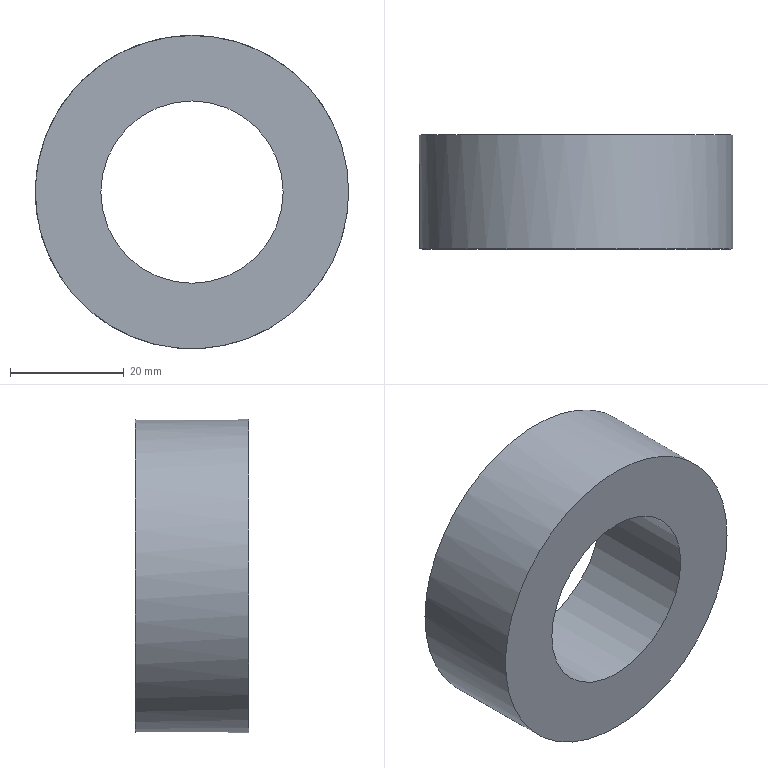Part | NX | features solid 2 | 1 solid | 4 faces | box 55 x 20 x 55 mm | volume 31432 mm3 | cylinder 2 | plane 2 | commonest cylinder face diameters 32 x1 55 x1
STEP:
#1=CARTESIAN_POINT('',(-594.,592.,-380.));
#2=VERTEX_POINT('',#1);
#3=CARTESIAN_POINT('',(-610.,592.,-380.));
#4=DIRECTION('',(0.,-1.,0.));
#5=DIRECTION('',(1.,0.,0.));
#6=AXIS2_PLACEMENT_3D('',#3,#4,#5);
#7=CIRCLE('',#6,16.);
#8=EDGE_CURVE('',#2,#2,#7,.T.);
#9=ORIENTED_EDGE('',*,*,#8,.F.);
#10=EDGE_LOOP('',(#9));
#11=FACE_BOUND('',#10,.T.);
#12=CARTESIAN_POINT('',(-610.,572.,-364.));
#13=VERTEX_POINT('',#12);
#14=CARTESIAN_POINT('',(-610.,572.,-380.));
#15=DIRECTION('',(0.,-1.,0.));
#16=DIRECTION('',(0.,0.,1.));
#17=AXIS2_PLACEMENT_3D('',#14,#15,#16);
#18=CIRCLE('',#17,16.);
#19=EDGE_CURVE('',#13,#13,#18,.T.);
#20=ORIENTED_EDGE('',*,*,#19,.T.);
#21=EDGE_LOOP('',(#20));
#22=FACE_BOUND('',#21,.T.);
#23=CARTESIAN_POINT('',(-610.,592.,-380.));
#24=DIRECTION('',(0.,-1.,0.));
#25=DIRECTION('',(1.,0.,0.));
#26=AXIS2_PLACEMENT_3D('',#23,#24,#25);
#27=CYLINDRICAL_SURFACE('',#26,16.);
#28=ADVANCED_FACE('',(#11,#22),#27,.F.);
#29=CARTESIAN_POINT('',(-582.5,592.,-380.));
#30=VERTEX_POINT('',#29);
#31=CARTESIAN_POINT('',(-610.,592.,-380.));
#32=DIRECTION('',(0.,-1.,0.));
#33=DIRECTION('',(1.,0.,0.));
#34=AXIS2_PLACEMENT_3D('',#31,#32,#33);
#35=CIRCLE('',#34,27.5);
#36=EDGE_CURVE('',#30,#30,#35,.T.);
#37=ORIENTED_EDGE('',*,*,#36,.T.);
#38=EDGE_LOOP('',(#37));
#39=FACE_BOUND('',#38,.T.);
#40=CARTESIAN_POINT('',(-610.,572.,-352.5));
#41=VERTEX_POINT('',#40);
#42=CARTESIAN_POINT('',(-610.,572.,-380.));
#43=DIRECTION('',(0.,-1.,0.));
#44=DIRECTION('',(0.,0.,1.));
#45=AXIS2_PLACEMENT_3D('',#42,#43,#44);
#46=CIRCLE('',#45,27.5);
#47=EDGE_CURVE('',#41,#41,#46,.T.);
#48=ORIENTED_EDGE('',*,*,#47,.F.);
#49=EDGE_LOOP('',(#48));
#50=FACE_BOUND('',#49,.T.);
#51=CARTESIAN_POINT('',(-610.,592.,-380.));
#52=DIRECTION('',(0.,-1.,0.));
#53=DIRECTION('',(1.,0.,0.));
#54=AXIS2_PLACEMENT_3D('',#51,#52,#53);
#55=CYLINDRICAL_SURFACE('',#54,27.5);
#56=ADVANCED_FACE('',(#39,#50),#55,.T.);
#57=ORIENTED_EDGE('',*,*,#8,.T.);
#58=EDGE_LOOP('',(#57));
#59=FACE_BOUND('',#58,.T.);
#60=ORIENTED_EDGE('',*,*,#36,.F.);
#61=EDGE_LOOP('',(#60));
#62=FACE_BOUND('',#61,.T.);
#63=CARTESIAN_POINT('',(-610.,592.,-380.));
#64=DIRECTION('',(0.,-1.,0.));
#65=DIRECTION('',(1.,0.,0.));
#66=AXIS2_PLACEMENT_3D('',#63,#64,#65);
#67=PLANE('',#66);
#68=ADVANCED_FACE('',(#59,#62),#67,.F.);
#69=ORIENTED_EDGE('',*,*,#19,.F.);
#70=EDGE_LOOP('',(#69));
#71=FACE_BOUND('',#70,.T.);
#72=ORIENTED_EDGE('',*,*,#47,.T.);
#73=EDGE_LOOP('',(#72));
#74=FACE_BOUND('',#73,.T.);
#75=CARTESIAN_POINT('',(-610.,572.,-380.));
#76=DIRECTION('',(0.,-1.,0.));
#77=DIRECTION('',(1.,0.,0.));
#78=AXIS2_PLACEMENT_3D('',#75,#76,#77);
#79=PLANE('',#78);
#80=ADVANCED_FACE('',(#71,#74),#79,.T.);
#81=CLOSED_SHELL('',(#28,#56,#68,#80));
#82=MANIFOLD_SOLID_BREP('',#81);
#83=(LENGTH_UNIT()NAMED_UNIT(*)SI_UNIT(.MILLI.,.METRE.));
#84=UNCERTAINTY_MEASURE_WITH_UNIT(LENGTH_MEASURE(0.00001),#83,'','');
#85=(NAMED_UNIT(*)PLANE_ANGLE_UNIT()SI_UNIT($,.RADIAN.));
#86=(NAMED_UNIT(*)SI_UNIT($,.STERADIAN.)SOLID_ANGLE_UNIT());
#87=(GEOMETRIC_REPRESENTATION_CONTEXT(3)GLOBAL_UNCERTAINTY_ASSIGNED_CONTEXT((#84))GLOBAL_UNIT_ASSIGNED_CONTEXT((#83,#85,#86))REPRESENTATION_CONTEXT('',''));
#88=ADVANCED_BREP_SHAPE_REPRESENTATION('',(#82),#87);